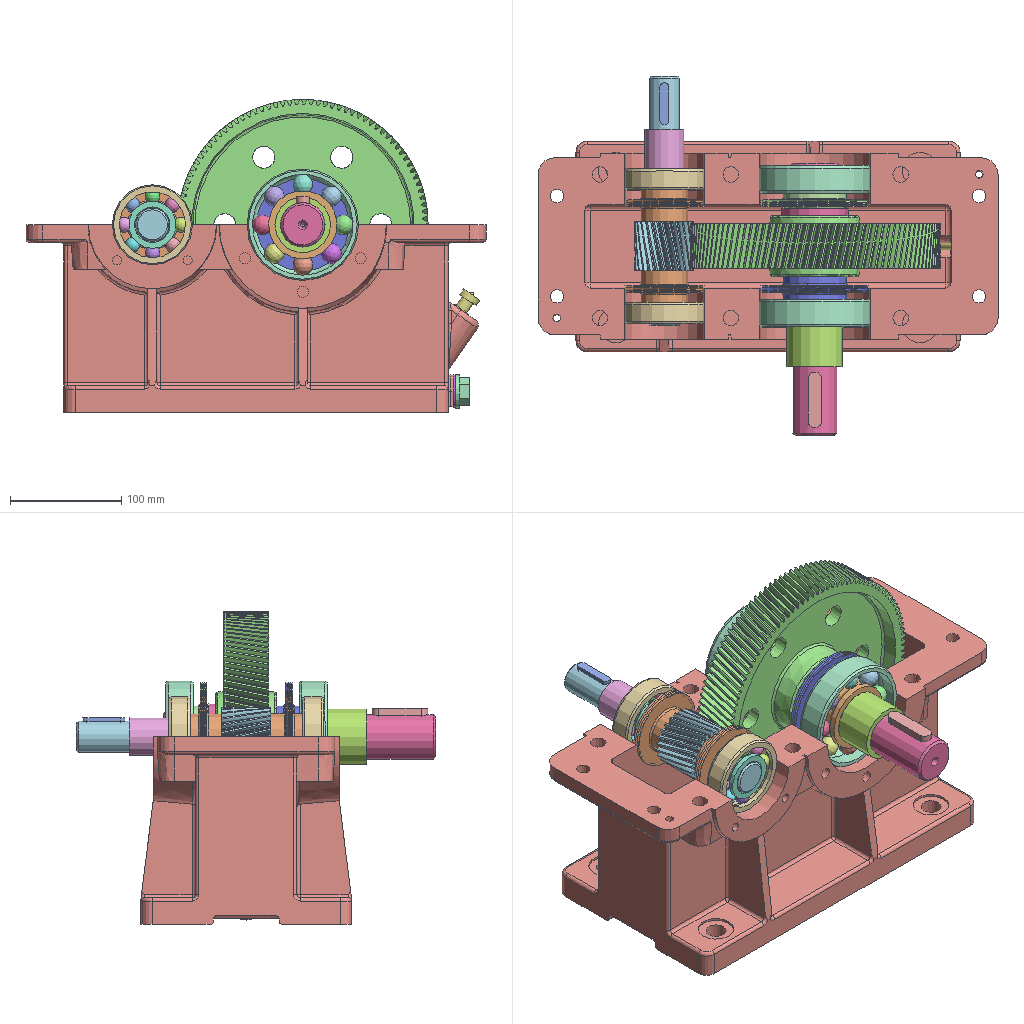Assembly | NX | 18 different items | 21 placed | box 413 x 322 x 281 mm
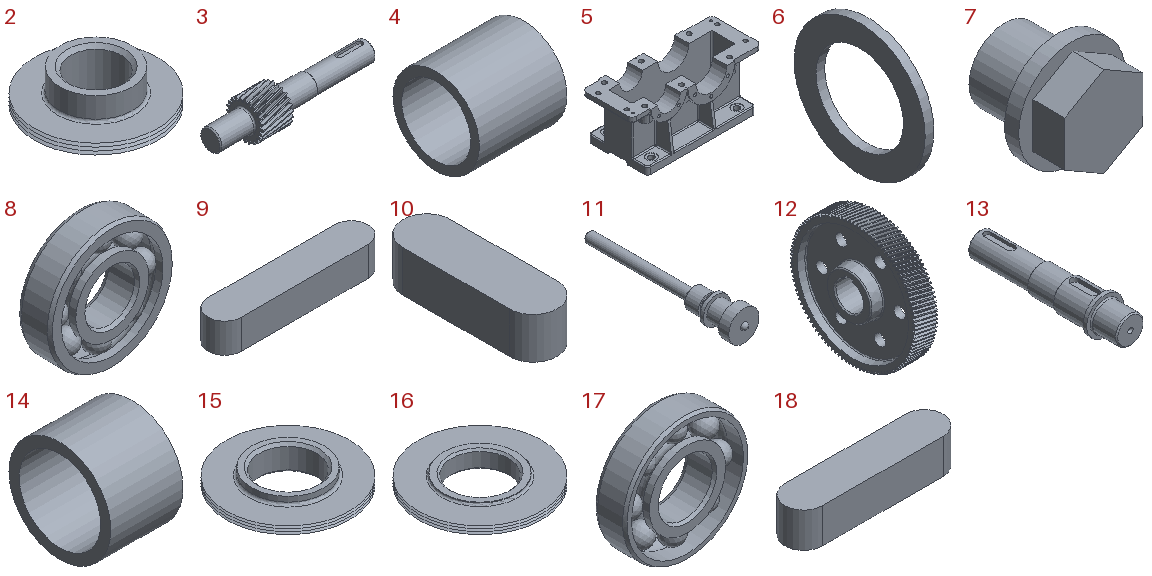Parts list (item | name | quantity | size | volume | features):
1 | 26. drain plug | x1 | - | - | -
2 | - | x2 | 72 x 72 x 28.5 mm | 34035 mm3 | features DATUM_CSYS 2, SKETCH 1, SWP104 1
3 | - | x1 | 223.5 x 53.091 x 53.091 mm | 200222 mm3 | features BREP 24, META 24, DATUM_CSYS 3, SKETCH 2, BLEND 1, CHAMFER 1, CYLINDER 1, EXTRUDE 1, FSET 1, SWP104 1
4 | - | x1 | 35.5 x 35 x 35 mm | 12296 mm3 | features DATUM_CSYS 2, EXTRUDE 1, SKETCH 1
5 | - | x1 | 413 x 189 x 168.5 mm | 3122750 mm3 | features DATUM_CSYS 38, SKETCH 37, EXTRUDE 25, EXTRACT_FACE 22, SIMPLE HOLE 10, Instance Feature 8, HOLE PACKAGE 7, Mirror Feature 5, CBORE_HOLE 4, CPROJ 4, EXTRACT_DATUM_PLANE 4, RIB 4, BLEND 3, DATUM_PLANE 2, TAPER_HOLE 2, Pattern Feature 1, UNITE 1
6 | - | x1 | 2 x 30 x 30 mm | 785.398 mm3 | features DATUM_CSYS 2, EXTRUDE 1, LINKED_FACE 1, SKETCH 1
7 | - | x1 | 30 x 28 x 30 mm | 11086 mm3 | features DATUM_CSYS 3, SKETCH 2, EXTRUDE 1, SWP104 1, SYMBOLIC_THREAD 1
8 | - | x2 | 72 x 19 x 72 mm | 39104 mm3 | features DATUM_CSYS 10, SKETCH 9, SWP104 9, EXTRACT_DATUM_AXIS 8, EXTRACT_DATUM_PLANE 8, EXTRACT_FACE 8, EXTRACT_STRING 8, Instance Feature 7, Pattern Feature 1
9 | - | x1 | 38 x 8 x 7 mm | 2032 mm3 | features DATUM_CSYS 2, EXTRUDE 1, SKETCH 1
10 | - | x1 | 14 x 45 x 12 mm | 7055 mm3 | features DATUM_CSYS 2, EXTRUDE 1, LINKED_FACE 1, SKETCH 1
11 | - | x1 | 18 x 94 x 18 mm | 6155 mm3 | features DATUM_CSYS 2, CHAMFER 1, SKETCH 1, SWP104 1, SYMBOLIC_THREAD 1
12 | - | x1 | 55 x 224.908 x 224.908 mm | 752856 mm3 | features BREP 108, META 108, DATUM_CSYS 9, EXTRUDE 8, SKETCH 8, EXTRACT_DATUM_AXIS 6, DRAFT 4, BLEND 2, CHAMFER 2, EXTRACT_DATUM_PLANE 2, EXTRACT_FACE 2, EXTRACT_STRING 2, CYLINDER 1, DATUM_PLANE 1, FSET 1, Instance Feature 1, Mirror Feature 1
13 | - | x1 | 60 x 244.5 x 60 mm | 375385 mm3 | features DATUM_CSYS 4, SKETCH 3, EXTRUDE 2, SWP104 1
14 | - | x1 | 35.5 x 50 x 50 mm | 25093 mm3 | features DATUM_CSYS 2, EXTRUDE 1, SKETCH 1
15 | - | x1 | 97 x 97 x 20 mm | 46420 mm3 | features DATUM_CSYS 2, SKETCH 1, SWP104 1
16 | - | x1 | 97 x 97 x 14 mm | 40772 mm3 | features DATUM_CSYS 2, SKETCH 1, SWP104 1
17 | - | x2 | 100 x 25 x 100 mm | 93926 mm3 | features DATUM_CSYS 10, SKETCH 9, SWP104 9, EXTRACT_DATUM_AXIS 8, EXTRACT_DATUM_PLANE 8, EXTRACT_STRING 8, Instance Feature 7, Pattern Feature 1
18 | - | x1 | 50 x 12 x 11 mm | 6260 mm3 | features DATUM_CSYS 2, EXTRUDE 1, SKETCH 1
Mates (type | each side: item.copy, entity, surface, feature):
Touch | 11.1 face cylinder Revolve(2) | 5.1 face cylinder Extrude(13)
Concentric | 11.1 edge | 5.1 edge
Fix | 5.1 component
Touch | 5.1 face cylinder Extrude(6) | 3.1 face cylinder Revolve(52)
Touch | 13.1 face cylinder Revolve(2) | 5.1 face cylinder Extrude(6)
Touch | 13.1 face cylinder Revolve(2) | 12.1 face cone Mirror Feature(227)
Center22 | 3.1 face plane Cylinder(1) | 3.1 face plane Cylinder(1) | 5.1 face plane Extrude(3) | 5.1 face plane Mirror Feature(5)
Center22 | 12.1 face plane Mirror Feature(227) | 12.1 face plane Extrude(219) | 5.1 face plane Extrude(4) | 5.1 face plane Mirror Feature(5)
Touch | 2.1 face cylinder Revolve(2) | 5.1 face cylinder Extrude(6)
Touch | 2.1 face plane Revolve(2) | 3.1 face plane Cylinder(1)
Touch | 5.1 face cylinder Extrude(6) | 2.1 face cylinder Revolve(2)
Touch | 3.1 face plane Cylinder(1) | 2.1 face plane Revolve(2)
Touch | 8.1 face cylinder Revolve(1) | 5.1 face cylinder Extrude(6)
Touch | 8.1 face plane Revolve(1) | 2.1 face plane Revolve(2)
Touch | 5.1 face cylinder Extrude(6) | 8.1 face cylinder Revolve(1)
Touch | 2.1 face plane Revolve(2) | 8.1 face plane Revolve(1)
Touch | 16.1 face cylinder Revolve(1) | 5.1 face cylinder Extrude(6)
Touch | 13.1 face plane Revolve(2) | 12.1 face plane Extrude(221)
Touch | 10.1 face cylinder Extrude(2) | 13.1 face cylinder Extrude(4)
Touch | 16.1 face plane Revolve(1) | 13.1 face plane Revolve(2)
Touch | 17.1 face cylinder Revolve(1) | 5.1 face cylinder Extrude(6) | 2 times
Touch | 17.1 face plane Revolve(1) | 16.1 face plane Revolve(1)
Touch | 15.1 face cylinder Revolve(2) | 5.1 face cylinder Extrude(6)
Touch | 15.1 face plane Revolve(2) | 12.1 face plane Mirror Feature(227)
Touch | 17.1 face plane Revolve(1) | 15.1 face plane Revolve(2)
Touch | 4.1 face cylinder Extrude(1) | 3.1 face cylinder Revolve(52)
Touch | 4.1 face plane Extrude(1) | 8.1 face plane Revolve(1)
Touch | 14.1 face cylinder Extrude(1) | 13.1 face cylinder Revolve(2)
Touch | 14.1 face plane Extrude(1) | 17.1 face plane Revolve(1)
Concentric | 9.1 edge | 3.1 edge | 2 times
Concentric | 18.1 edge | 13.1 edge | 2 times